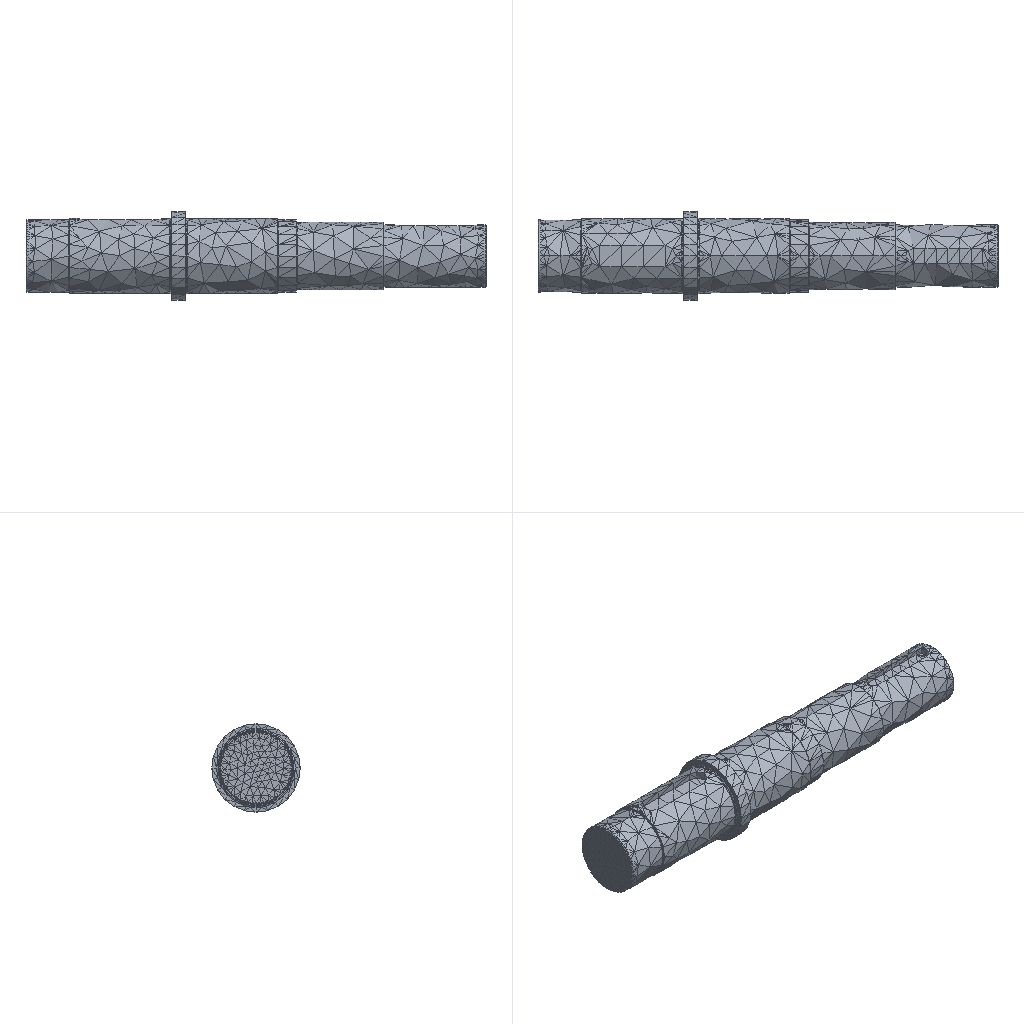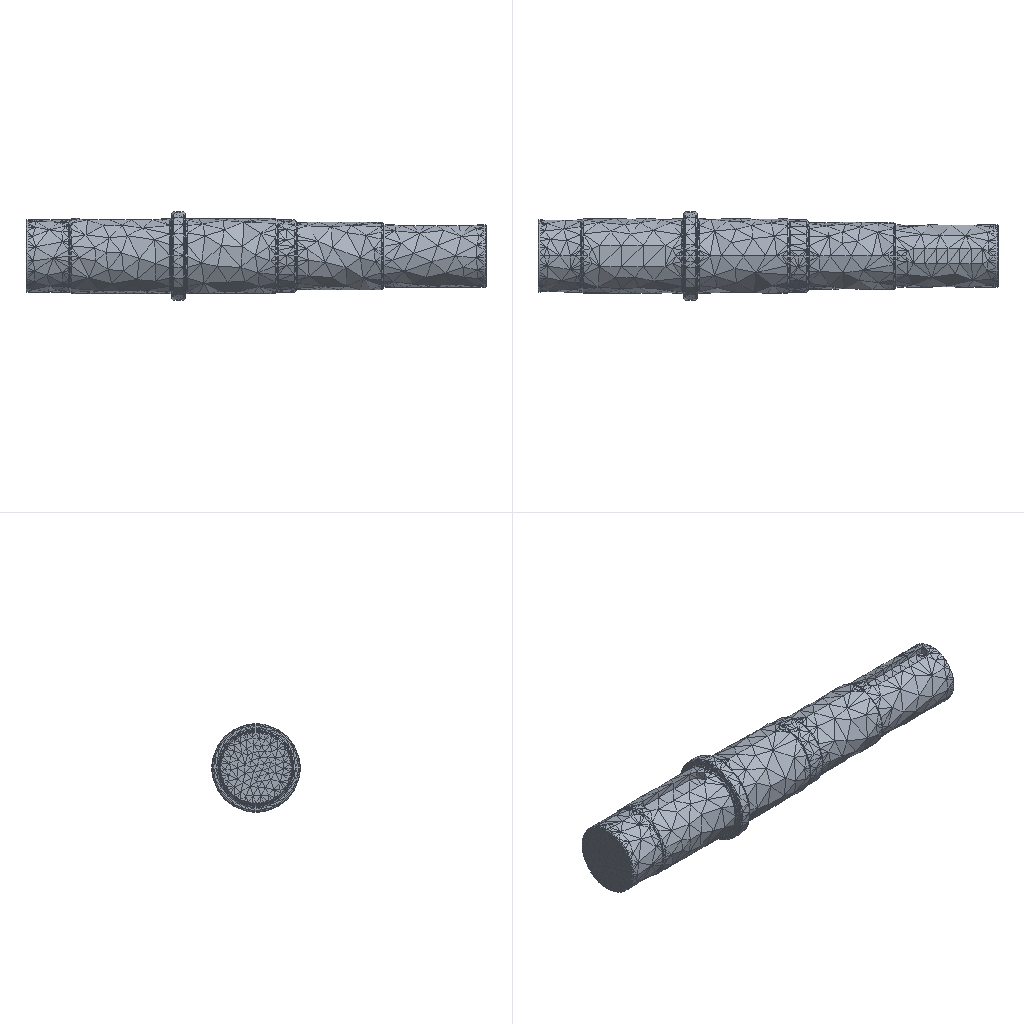Simulation study | ansys workbench
Set-up summary:
category,name,step,type,value,unit,region
solver,ansys_mapdl
solver,version,,,22.1
solver,version,,,22.1
units,MPA,,stated
analysis,deck1,,static,static
load_step,requested,,,1
analysis,nlgeom,,,False
mesh,nodes,,,13448
mesh,elements,,,8169
element_type,ANSYS 187 (type 1),,solid,7656
element_type,ANSYS 174 (type 2),,contact,513
element_type,ANSYS 170 (type 3),,target,0
load,load commands in deck,,count,3
bc,support commands in deck,,count,1
named_set,_FIXEDSU,,component
analysis,deck2,,static,static
load_step,requested,,,1
analysis,nlgeom,,,False
mesh,nodes,,,11812
mesh,elements,,,7175
element_type,ANSYS 187 (type 1),,solid,6720
element_type,ANSYS 174 (type 2),,contact,455
element_type,ANSYS 170 (type 3),,target,0
load,load commands in deck,,count,3
bc,support commands in deck,,count,1
named_set,_FIXEDSU,,component
material,1,,in results
material,1,,in results
check,setup vs results,,match,results also hold 0 node(s) and 1 element(s) the deck makes with ['EN']; those were not compared; 1 node(s) the solver created internally for pilot nodes (ansys-fenxi-4/轴有限元分析222/1_files/dp0/SYS-1/MECH/solve.out) are in the results only
check,setup vs results,,match,results also hold 0 node(s) and 1 element(s) the deck makes with ['EN']; those were not compared; 1 node(s) the solver created internally for pilot nodes (ansys-fenxi-4/轴有限元分析222/1_files/dp0/SYS/MECH/solve.out) are in the results only
Results summary:
result,analysis,,,static
result,last_loadstep,,,1
result,primary field,,,displacement
result,reaction total,1,FX,3.2e-05,N
result,reaction total,1,FY,-1.2e-05,N
result,reaction total,1,FZ,7e-06,N
result,mass,,,0.01585,"NMM: mm, ton, N, s, mV, mA, degC"
result,analysis,,,static
result,last_loadstep,,,1
result,primary field,,,displacement
result,reaction total,1,FX,1.8e-05,N
result,reaction total,1,FY,1e-05,N
result,reaction total,1,FZ,5e-06,N
result,mass,,,0.01586,"NMM: mm, ton, N, s, mV, mA, degC"